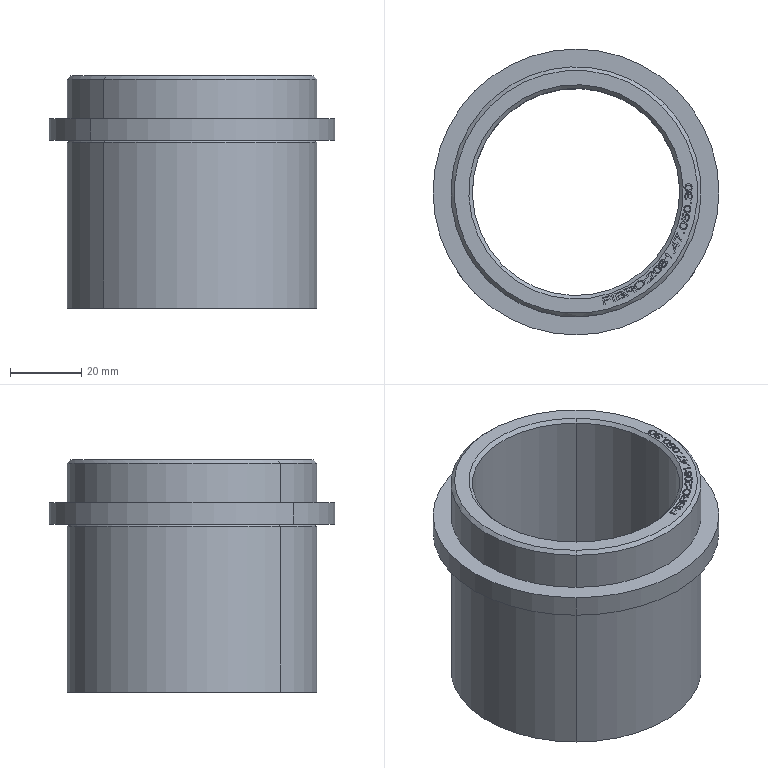Part | NX | features 1 2 | 1 solid | 244 faces | box 80 x 80 x 65 mm | volume 84989 mm3 | plane 122 | spline 104 | cylinder 8 | cone 6 | torus 4 | commonest cylinder face diameters 70 x4 58 x2 80 x2